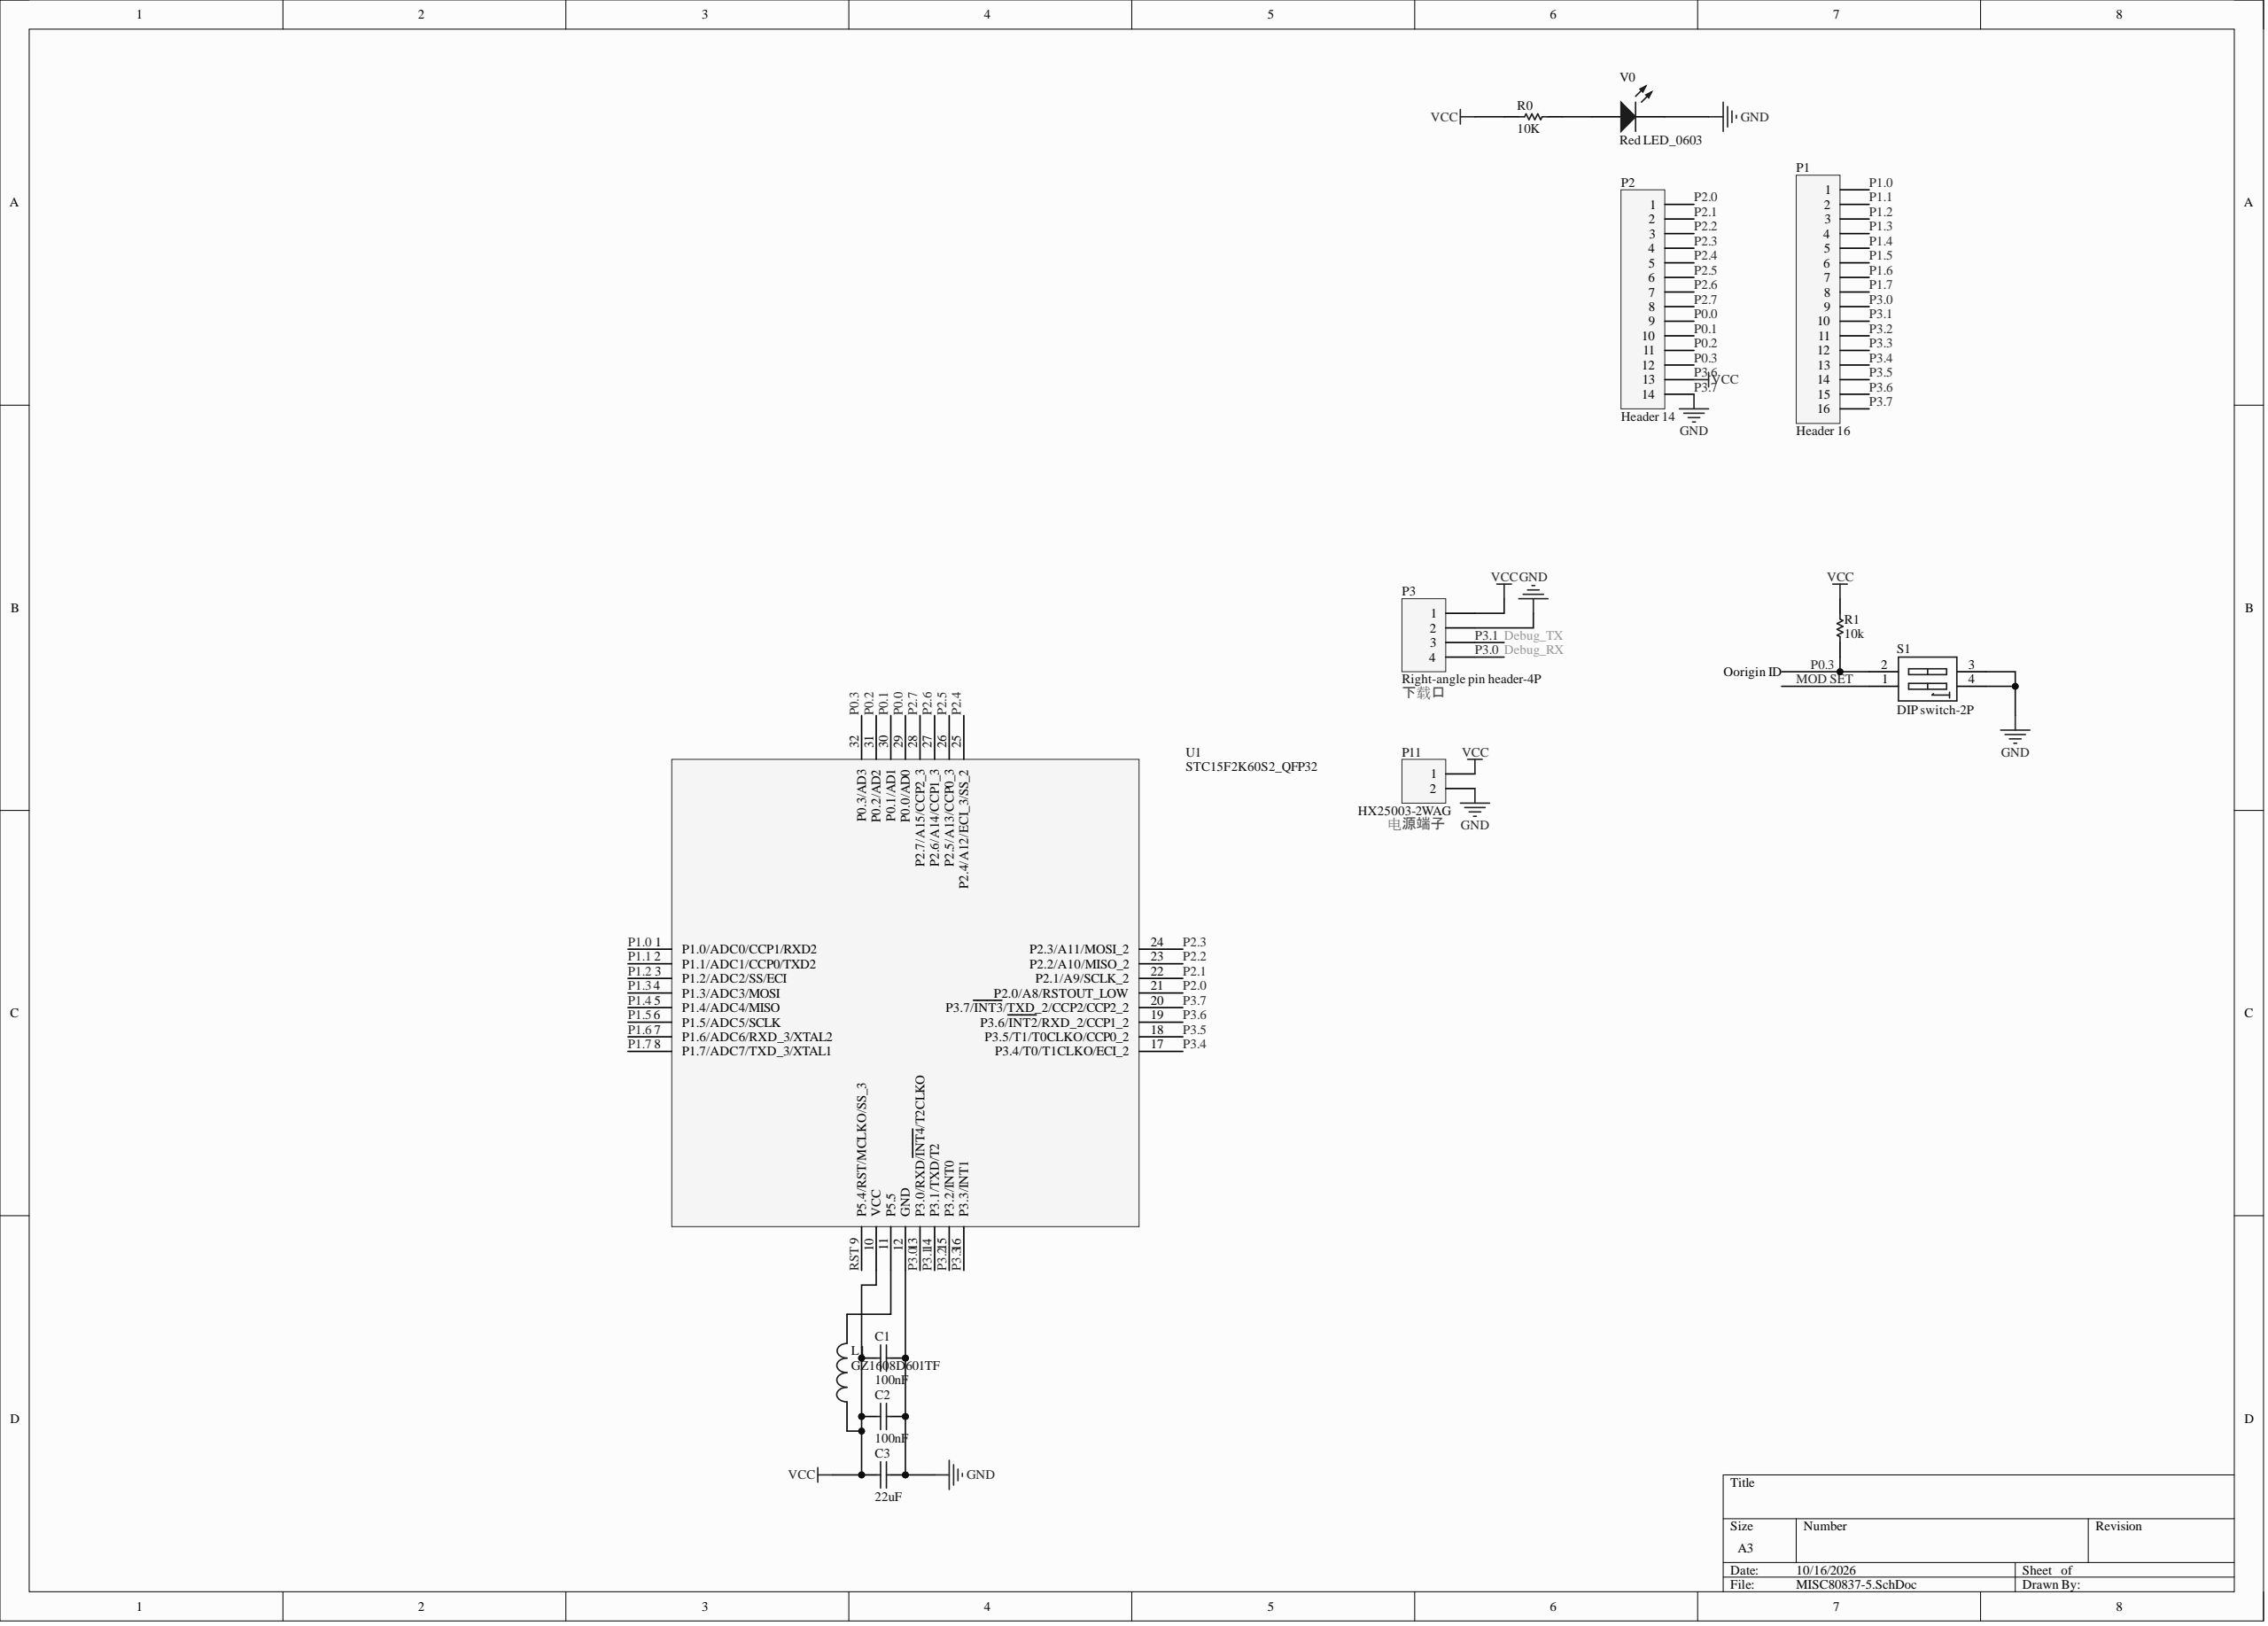Circuit board | Altium Designer | 13 parts | 30 nets
Bill of materials:
Comment,Description,Designator,Footprint,LibRef,Quantity
"100nF","Non-polarized capacitor","C1, C2","C0603","CAP","2"
"22uF","Non-polarized capacitor","C3","C0603","CAP","1"
"GZ1608D601TF","INDUCTOR","L1","AL0204","INDUCTOR","1"
"Header 16","Header, 16-Pin","P1","HDR1X16","Header 16","1"
"Header 14","Header, 14-Pin","P2","HDR1X14","Header 14","1"
"Right-angle pin header-4P","Header, 4-Pin","P3","HDR1X4","Header 4","1"
"HX25003-2WAG","Header, 2-Pin, Right Angle","P11","HDR1X2","Header 2H","1"
"10K","","R0, R1","6-0805_N","RES","2"
"DIP switch-2P","DIP Switch, 2 Position, SPST","S1","DIP-4","SW DIP-2","1"
"STC15F2K60S2_QFP32","","U1","LQFP32","STC15F2K60S2_QFP32","1"
"Red LED_0603","Typical RED GaAs LED","V0","3.2X1.6X1.1","LED1","1"
Netlist (Protel format):
[
C1
C0603
100nF



]
[
C2
C0603
100nF



]
[
C3
C0603
22uF



]
[
L1
AL0204
GZ1608D601TF



]
[
P1
HDR1X16
Header 16



]
[
P2
HDR1X14
Header 14



]
[
P3
HDR1X4
Right-angle pin header-4P



]
[
P11
HDR1X2
HX25003-2WAG



]
[
R0
6-0805_N
10K



]
[
R1
6-0805_N
10k



]
[
S1
DIP-4
DIP switch-2P



]
[
U1
LQFP32
STC15F2K60S2_QFP32



]
[
V0
3.2X1.6X1.1
Red LED_0603



]
(
P3.7
C1-1
C2-1
C3-1
P1-16
P2-14
P3-2
P11-2
S1-3
S1-4
U1-12
U1-20
V0-2
)
(
P3.6
C1-2
C2-2
C3-2
L1-1
P1-15
P2-13
P3-1
P11-1
R0-1
R1-2
U1-10
U1-19
)
(
P3.5
P1-14
U1-18
)
(
P3.4
P1-13
U1-17
)
(
P3.3
P1-12
U1-16
)
(
P3.2
P1-11
U1-15
)
(
P2.7
P2-8
U1-28
)
(
P2.6
P2-7
U1-27
)
(
P2.5
P2-6
U1-26
)
(
P2.4
P2-5
U1-25
)
(
P2.3
P2-4
U1-24
)
(
P2.2
P2-3
U1-23
)
(
P2.1
P2-2
U1-22
)
(
P2.0
P2-1
U1-21
)
(
P1.7
P1-8
U1-8
)
(
P1.6
P1-7
U1-7
)
(
P1.5
P1-6
U1-6
)
(
P1.4
P1-5
U1-5
)
(
P1.3
P1-4
U1-4
)
(
P1.2
P1-3
U1-3
)
(
P1.1
P1-2
U1-2
)
(
P1.0
P1-1
U1-1
)
(
P0.2
P2-11
U1-31
)
(
P0.1
P2-10
U1-30
)
(
P0.0
P2-9
U1-29
)
(
Oorigin ID
P2-12
R1-1
S1-2
U1-32
)
(
NetR0_2
R0-2
V0-1
)
(
NetL1_2
L1-2
U1-11
)
(
Debug_TX
P1-10
P3-3
U1-14
)
(
Debug_RX
P1-9
P3-4
U1-13
)